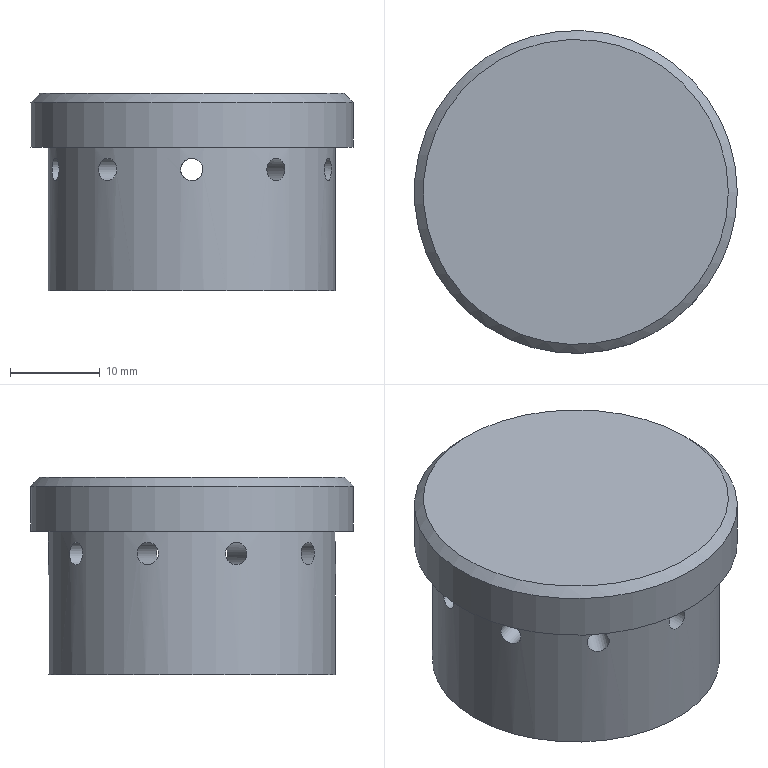Part | NX | features EXTRUDE 12, EXTRACT_STRING 10, Instance Feature 9, DATUM_CSYS 4, SKETCH 3, BOSS 1, CHAMFER 1, CYLINDER 1, Pattern Feature 1 | 1 solid | 20 faces | box 36 x 36 x 22 mm | volume 11377 mm3 | cylinder 14 | plane 5 | cone 1 | commonest cylinder face diameters 2.5 x10 18 x1 25 x1 32 x1 36 x1
STEP:
#1=CARTESIAN_POINT('',(-15.557,-3.74,13.5));
#2=VERTEX_POINT('',#1);
#3=CARTESIAN_POINT('',(-15.496,-4.006,12.519));
#4=CARTESIAN_POINT('',(-15.587,-3.608,13.5));
#5=CARTESIAN_POINT('',(-15.496,-4.006,14.48));
#6=CARTESIAN_POINT('',(-15.229,-4.947,14.885));
#7=CARTESIAN_POINT('',(-14.891,-5.868,14.48));
#8=CARTESIAN_POINT('',(-14.731,-6.243,13.5));
#9=CARTESIAN_POINT('',(-14.891,-5.869,12.522));
#10=CARTESIAN_POINT('',(-15.228,-4.949,12.115));
#11=CARTESIAN_POINT('',(-15.496,-4.006,12.519));
#12=CARTESIAN_POINT('',(-15.587,-3.608,13.5));
#13=CARTESIAN_POINT('',(-15.496,-4.006,14.48));
#14=B_SPLINE_CURVE_WITH_KNOTS('',3,(#3,#4,#5,#6,#7,#8,#9,#10,#11,#12,#13),.UNSPECIFIED.,.T.,.F.,(1,1,1,1,1,1,1,1,1,1,1,1,1,1,1),(-0.002932,-0.001955,-0.0009773,0.,0.0009773,0.001955,0.002932,0.003909,0.004886,0.005864,0.006841,0.007818,0.008795,0.009773,0.01075),.UNSPECIFIED.);
#15=EDGE_CURVE('',#2,#2,#14,.T.);
#16=ORIENTED_EDGE('',*,*,#15,.T.);
#17=EDGE_LOOP('',(#16));
#18=FACE_BOUND('',#17,.T.);
#19=CARTESIAN_POINT('',(-8.365,13.639,13.5));
#20=VERTEX_POINT('',#19);
#21=CARTESIAN_POINT('',(-8.598,13.5,12.519));
#22=CARTESIAN_POINT('',(-8.248,13.709,13.5));
#23=CARTESIAN_POINT('',(-8.598,13.5,14.48));
#24=CARTESIAN_POINT('',(-9.411,12.955,14.885));
#25=CARTESIAN_POINT('',(-10.182,12.349,14.48));
#26=CARTESIAN_POINT('',(-10.489,12.081,13.5));
#27=CARTESIAN_POINT('',(-10.183,12.348,12.522));
#28=CARTESIAN_POINT('',(-9.413,12.953,12.115));
#29=CARTESIAN_POINT('',(-8.598,13.5,12.519));
#30=CARTESIAN_POINT('',(-8.248,13.709,13.5));
#31=CARTESIAN_POINT('',(-8.598,13.5,14.48));
#32=B_SPLINE_CURVE_WITH_KNOTS('',3,(#21,#22,#23,#24,#25,#26,#27,#28,#29,#30,#31),.UNSPECIFIED.,.T.,.F.,(1,1,1,1,1,1,1,1,1,1,1,1,1,1,1),(-0.002932,-0.001955,-0.0009773,0.,0.0009773,0.001955,0.002932,0.003909,0.004886,0.005864,0.006841,0.007818,0.008795,0.009773,0.01075),.UNSPECIFIED.);
#33=EDGE_CURVE('',#20,#20,#32,.T.);
#34=ORIENTED_EDGE('',*,*,#33,.T.);
#35=EDGE_LOOP('',(#34));
#36=FACE_BOUND('',#35,.T.);
#37=CARTESIAN_POINT('',(10.387,12.17,13.5));
#38=VERTEX_POINT('',#37);
#39=CARTESIAN_POINT('',(10.182,12.349,12.519));
#40=CARTESIAN_POINT('',(10.49,12.08,13.5));
#41=CARTESIAN_POINT('',(10.182,12.349,14.48));
#42=CARTESIAN_POINT('',(9.413,12.954,14.885));
#43=CARTESIAN_POINT('',(8.598,13.5,14.48));
#44=CARTESIAN_POINT('',(8.248,13.709,13.5));
#45=CARTESIAN_POINT('',(8.597,13.501,12.522));
#46=CARTESIAN_POINT('',(9.411,12.955,12.115));
#47=CARTESIAN_POINT('',(10.182,12.349,12.519));
#48=CARTESIAN_POINT('',(10.49,12.08,13.5));
#49=CARTESIAN_POINT('',(10.182,12.349,14.48));
#50=B_SPLINE_CURVE_WITH_KNOTS('',3,(#39,#40,#41,#42,#43,#44,#45,#46,#47,#48,#49),.UNSPECIFIED.,.T.,.F.,(1,1,1,1,1,1,1,1,1,1,1,1,1,1,1),(-0.002932,-0.001955,-0.0009773,0.,0.0009773,0.001955,0.002932,0.003909,0.004886,0.005864,0.006841,0.007818,0.008795,0.009773,0.01075),.UNSPECIFIED.);
#51=EDGE_CURVE('',#38,#38,#50,.T.);
#52=ORIENTED_EDGE('',*,*,#51,.T.);
#53=EDGE_LOOP('',(#52));
#54=FACE_BOUND('',#53,.T.);
#55=CARTESIAN_POINT('',(14.784,-6.118,13.5));
#56=VERTEX_POINT('',#55);
#57=CARTESIAN_POINT('',(14.891,-5.868,12.519));
#58=CARTESIAN_POINT('',(14.731,-6.243,13.5));
#59=CARTESIAN_POINT('',(14.891,-5.868,14.48));
#60=CARTESIAN_POINT('',(15.228,-4.949,14.885));
#61=CARTESIAN_POINT('',(15.496,-4.005,14.48));
#62=CARTESIAN_POINT('',(15.587,-3.608,13.5));
#63=CARTESIAN_POINT('',(15.497,-4.004,12.522));
#64=CARTESIAN_POINT('',(15.229,-4.947,12.115));
#65=CARTESIAN_POINT('',(14.891,-5.868,12.519));
#66=CARTESIAN_POINT('',(14.731,-6.243,13.5));
#67=CARTESIAN_POINT('',(14.891,-5.868,14.48));
#68=B_SPLINE_CURVE_WITH_KNOTS('',3,(#57,#58,#59,#60,#61,#62,#63,#64,#65,#66,#67),.UNSPECIFIED.,.T.,.F.,(1,1,1,1,1,1,1,1,1,1,1,1,1,1,1),(-0.002932,-0.001955,-0.0009773,0.,0.0009773,0.001955,0.002932,0.003909,0.004886,0.005864,0.006841,0.007818,0.008795,0.009773,0.01075),.UNSPECIFIED.);
#69=EDGE_CURVE('',#56,#56,#68,.T.);
#70=ORIENTED_EDGE('',*,*,#69,.T.);
#71=EDGE_LOOP('',(#70));
#72=FACE_BOUND('',#71,.T.);
#73=CARTESIAN_POINT('',(0.,-16.,14.75));
#74=VERTEX_POINT('',#73);
#75=CARTESIAN_POINT('',(-0.9806,-15.976,14.479));
#76=CARTESIAN_POINT('',(0.000248,-16.012,14.886));
#77=CARTESIAN_POINT('',(0.9796,-15.976,14.479));
#78=CARTESIAN_POINT('',(1.385,-15.939,13.501));
#79=CARTESIAN_POINT('',(0.9801,-15.976,12.521));
#80=CARTESIAN_POINT('',(0.0002185,-16.012,12.115));
#81=CARTESIAN_POINT('',(-0.9783,-15.976,12.52));
#82=CARTESIAN_POINT('',(-1.385,-15.939,13.499));
#83=CARTESIAN_POINT('',(-0.9806,-15.976,14.479));
#84=CARTESIAN_POINT('',(0.000248,-16.012,14.886));
#85=CARTESIAN_POINT('',(0.9796,-15.976,14.479));
#86=B_SPLINE_CURVE_WITH_KNOTS('',3,(#75,#76,#77,#78,#79,#80,#81,#82,#83,#84,#85),.UNSPECIFIED.,.T.,.F.,(1,1,1,1,1,1,1,1,1,1,1,1,1,1,1),(-0.002932,-0.001955,-0.0009773,0.,0.0009773,0.001955,0.002932,0.003909,0.004886,0.005864,0.006841,0.007818,0.008795,0.009773,0.01075),.UNSPECIFIED.);
#87=EDGE_CURVE('',#74,#74,#86,.T.);
#88=ORIENTED_EDGE('',*,*,#87,.T.);
#89=EDGE_LOOP('',(#88));
#90=FACE_BOUND('',#89,.T.);
#91=CARTESIAN_POINT('',(16.,0.,16.));
#92=VERTEX_POINT('',#91);
#93=CARTESIAN_POINT('',(0.,0.,16.));
#94=DIRECTION('',(0.,0.,-1.));
#95=DIRECTION('',(1.,0.,0.));
#96=AXIS2_PLACEMENT_3D('',#93,#94,#95);
#97=CIRCLE('',#96,16.);
#98=EDGE_CURVE('',#92,#92,#97,.T.);
#99=ORIENTED_EDGE('',*,*,#98,.T.);
#100=EDGE_LOOP('',(#99));
#101=FACE_BOUND('',#100,.T.);
#102=CARTESIAN_POINT('',(16.,0.,0.));
#103=VERTEX_POINT('',#102);
#104=CARTESIAN_POINT('',(0.,0.,0.));
#105=DIRECTION('',(0.,0.,1.));
#106=DIRECTION('',(1.,0.,0.));
#107=AXIS2_PLACEMENT_3D('',#104,#105,#106);
#108=CIRCLE('',#107,16.);
#109=EDGE_CURVE('',#103,#103,#108,.T.);
#110=ORIENTED_EDGE('',*,*,#109,.T.);
#111=EDGE_LOOP('',(#110));
#112=FACE_BOUND('',#111,.T.);
#113=CARTESIAN_POINT('',(8.365,-13.639,13.5));
#114=VERTEX_POINT('',#113);
#115=CARTESIAN_POINT('',(8.598,-13.5,12.519));
#116=CARTESIAN_POINT('',(8.248,-13.709,13.5));
#117=CARTESIAN_POINT('',(8.598,-13.5,14.48));
#118=CARTESIAN_POINT('',(9.411,-12.955,14.885));
#119=CARTESIAN_POINT('',(10.182,-12.349,14.48));
#120=CARTESIAN_POINT('',(10.489,-12.081,13.5));
#121=CARTESIAN_POINT('',(10.183,-12.348,12.522));
#122=CARTESIAN_POINT('',(9.413,-12.953,12.115));
#123=CARTESIAN_POINT('',(8.598,-13.5,12.519));
#124=CARTESIAN_POINT('',(8.248,-13.709,13.5));
#125=CARTESIAN_POINT('',(8.598,-13.5,14.48));
#126=B_SPLINE_CURVE_WITH_KNOTS('',3,(#115,#116,#117,#118,#119,#120,#121,#122,#123,#124,#125),.UNSPECIFIED.,.T.,.F.,(1,1,1,1,1,1,1,1,1,1,1,1,1,1,1),(-0.002932,-0.001955,-0.0009773,0.,0.0009773,0.001955,0.002932,0.003909,0.004886,0.005864,0.006841,0.007818,0.008795,0.009773,0.01075),.UNSPECIFIED.);
#127=EDGE_CURVE('',#114,#114,#126,.T.);
#128=ORIENTED_EDGE('',*,*,#127,.T.);
#129=EDGE_LOOP('',(#128));
#130=FACE_BOUND('',#129,.T.);
#131=CARTESIAN_POINT('',(15.557,3.74,13.5));
#132=VERTEX_POINT('',#131);
#133=CARTESIAN_POINT('',(15.496,4.006,12.519));
#134=CARTESIAN_POINT('',(15.587,3.608,13.5));
#135=CARTESIAN_POINT('',(15.496,4.006,14.48));
#136=CARTESIAN_POINT('',(15.229,4.947,14.885));
#137=CARTESIAN_POINT('',(14.891,5.868,14.48));
#138=CARTESIAN_POINT('',(14.731,6.243,13.5));
#139=CARTESIAN_POINT('',(14.891,5.869,12.522));
#140=CARTESIAN_POINT('',(15.228,4.949,12.115));
#141=CARTESIAN_POINT('',(15.496,4.006,12.519));
#142=CARTESIAN_POINT('',(15.587,3.608,13.5));
#143=CARTESIAN_POINT('',(15.496,4.006,14.48));
#144=B_SPLINE_CURVE_WITH_KNOTS('',3,(#133,#134,#135,#136,#137,#138,#139,#140,#141,#142,#143),.UNSPECIFIED.,.T.,.F.,(1,1,1,1,1,1,1,1,1,1,1,1,1,1,1),(-0.002932,-0.001955,-0.0009773,0.,0.0009773,0.001955,0.002932,0.003909,0.004886,0.005864,0.006841,0.007818,0.008795,0.009773,0.01075),.UNSPECIFIED.);
#145=EDGE_CURVE('',#132,#132,#144,.T.);
#146=ORIENTED_EDGE('',*,*,#145,.T.);
#147=EDGE_LOOP('',(#146));
#148=FACE_BOUND('',#147,.T.);
#149=CARTESIAN_POINT('',(1.25,15.951,13.5));
#150=VERTEX_POINT('',#149);
#151=CARTESIAN_POINT('',(0.9787,15.976,12.519));
#152=CARTESIAN_POINT('',(1.386,15.939,13.5));
#153=CARTESIAN_POINT('',(0.979,15.976,14.48));
#154=CARTESIAN_POINT('',(0.001053,16.012,14.885));
#155=CARTESIAN_POINT('',(-0.9792,15.976,14.48));
#156=CARTESIAN_POINT('',(-1.385,15.939,13.5));
#157=CARTESIAN_POINT('',(-0.9805,15.976,12.522));
#158=CARTESIAN_POINT('',(-0.001401,16.012,12.115));
#159=CARTESIAN_POINT('',(0.9787,15.976,12.519));
#160=CARTESIAN_POINT('',(1.386,15.939,13.5));
#161=CARTESIAN_POINT('',(0.979,15.976,14.48));
#162=B_SPLINE_CURVE_WITH_KNOTS('',3,(#151,#152,#153,#154,#155,#156,#157,#158,#159,#160,#161),.UNSPECIFIED.,.T.,.F.,(1,1,1,1,1,1,1,1,1,1,1,1,1,1,1),(-0.002932,-0.001955,-0.0009773,0.,0.0009773,0.001955,0.002932,0.003909,0.004886,0.005864,0.006841,0.007818,0.008795,0.009773,0.01075),.UNSPECIFIED.);
#163=EDGE_CURVE('',#150,#150,#162,.T.);
#164=ORIENTED_EDGE('',*,*,#163,.T.);
#165=EDGE_LOOP('',(#164));
#166=FACE_BOUND('',#165,.T.);
#167=CARTESIAN_POINT('',(-14.784,6.118,13.5));
#168=VERTEX_POINT('',#167);
#169=CARTESIAN_POINT('',(-14.891,5.868,12.519));
#170=CARTESIAN_POINT('',(-14.731,6.243,13.5));
#171=CARTESIAN_POINT('',(-14.891,5.868,14.48));
#172=CARTESIAN_POINT('',(-15.228,4.949,14.885));
#173=CARTESIAN_POINT('',(-15.496,4.005,14.48));
#174=CARTESIAN_POINT('',(-15.587,3.608,13.5));
#175=CARTESIAN_POINT('',(-15.497,4.004,12.522));
#176=CARTESIAN_POINT('',(-15.229,4.947,12.115));
#177=CARTESIAN_POINT('',(-14.891,5.868,12.519));
#178=CARTESIAN_POINT('',(-14.731,6.243,13.5));
#179=CARTESIAN_POINT('',(-14.891,5.868,14.48));
#180=B_SPLINE_CURVE_WITH_KNOTS('',3,(#169,#170,#171,#172,#173,#174,#175,#176,#177,#178,#179),.UNSPECIFIED.,.T.,.F.,(1,1,1,1,1,1,1,1,1,1,1,1,1,1,1),(-0.002932,-0.001955,-0.0009773,0.,0.0009773,0.001955,0.002932,0.003909,0.004886,0.005864,0.006841,0.007818,0.008795,0.009773,0.01075),.UNSPECIFIED.);
#181=EDGE_CURVE('',#168,#168,#180,.T.);
#182=ORIENTED_EDGE('',*,*,#181,.T.);
#183=EDGE_LOOP('',(#182));
#184=FACE_BOUND('',#183,.T.);
#185=CARTESIAN_POINT('',(-10.387,-12.17,13.5));
#186=VERTEX_POINT('',#185);
#187=CARTESIAN_POINT('',(-10.182,-12.349,12.519));
#188=CARTESIAN_POINT('',(-10.49,-12.08,13.5));
#189=CARTESIAN_POINT('',(-10.182,-12.349,14.48));
#190=CARTESIAN_POINT('',(-9.413,-12.954,14.885));
#191=CARTESIAN_POINT('',(-8.598,-13.5,14.48));
#192=CARTESIAN_POINT('',(-8.248,-13.709,13.5));
#193=CARTESIAN_POINT('',(-8.597,-13.501,12.522));
#194=CARTESIAN_POINT('',(-9.411,-12.955,12.115));
#195=CARTESIAN_POINT('',(-10.182,-12.349,12.519));
#196=CARTESIAN_POINT('',(-10.49,-12.08,13.5));
#197=CARTESIAN_POINT('',(-10.182,-12.349,14.48));
#198=B_SPLINE_CURVE_WITH_KNOTS('',3,(#187,#188,#189,#190,#191,#192,#193,#194,#195,#196,#197),.UNSPECIFIED.,.T.,.F.,(1,1,1,1,1,1,1,1,1,1,1,1,1,1,1),(-0.002932,-0.001955,-0.0009773,0.,0.0009773,0.001955,0.002932,0.003909,0.004886,0.005864,0.006841,0.007818,0.008795,0.009773,0.01075),.UNSPECIFIED.);
#199=EDGE_CURVE('',#186,#186,#198,.T.);
#200=ORIENTED_EDGE('',*,*,#199,.T.);
#201=EDGE_LOOP('',(#200));
#202=FACE_BOUND('',#201,.T.);
#203=CARTESIAN_POINT('',(0.,0.,0.));
#204=DIRECTION('',(0.,0.,1.));
#205=DIRECTION('',(1.,0.,0.));
#206=AXIS2_PLACEMENT_3D('',#203,#204,#205);
#207=CYLINDRICAL_SURFACE('',#206,16.);
#208=ADVANCED_FACE('',(#18,#36,#54,#72,#90,#101,#112,#130,#148,#166,#184,#202),#207,.T.);
#209=CARTESIAN_POINT('',(-8.863,-1.565,13.5));
#210=VERTEX_POINT('',#209);
#211=CARTESIAN_POINT('',(-8.821,-1.837,14.481));
#212=CARTESIAN_POINT('',(-8.884,-1.43,13.5));
#213=CARTESIAN_POINT('',(-8.821,-1.837,12.52));
#214=CARTESIAN_POINT('',(-8.58,-2.787,12.115));
#215=CARTESIAN_POINT('',(-8.216,-3.699,12.52));
#216=CARTESIAN_POINT('',(-8.028,-4.065,13.5));
#217=CARTESIAN_POINT('',(-8.215,-3.7,14.478));
#218=CARTESIAN_POINT('',(-8.58,-2.789,14.885));
#219=CARTESIAN_POINT('',(-8.821,-1.837,14.481));
#220=CARTESIAN_POINT('',(-8.884,-1.43,13.5));
#221=CARTESIAN_POINT('',(-8.821,-1.837,12.52));
#222=B_SPLINE_CURVE_WITH_KNOTS('',3,(#211,#212,#213,#214,#215,#216,#217,#218,#219,#220,#221),.UNSPECIFIED.,.T.,.F.,(1,1,1,1,1,1,1,1,1,1,1,1,1,1,1),(-0.002934,-0.001956,-0.0009781,0.,0.0009781,0.001956,0.002934,0.003912,0.00489,0.005868,0.006847,0.007825,0.008803,0.009781,0.01076),.UNSPECIFIED.);
#223=EDGE_CURVE('',#210,#210,#222,.T.);
#224=ORIENTED_EDGE('',*,*,#223,.T.);
#225=EDGE_LOOP('',(#224));
#226=FACE_BOUND('',#225,.T.);
#227=CARTESIAN_POINT('',(-4.228,7.945,13.5));
#228=VERTEX_POINT('',#227);
#229=CARTESIAN_POINT('',(-4.473,7.821,14.481));
#230=CARTESIAN_POINT('',(-4.105,8.007,13.5));
#231=CARTESIAN_POINT('',(-4.473,7.822,12.52));
#232=CARTESIAN_POINT('',(-5.302,7.299,12.115));
#233=CARTESIAN_POINT('',(-6.057,6.67,12.52));
#234=CARTESIAN_POINT('',(-6.346,6.379,13.5));
#235=CARTESIAN_POINT('',(-6.058,6.67,14.478));
#236=CARTESIAN_POINT('',(-5.304,7.298,14.885));
#237=CARTESIAN_POINT('',(-4.473,7.821,14.481));
#238=CARTESIAN_POINT('',(-4.105,8.007,13.5));
#239=CARTESIAN_POINT('',(-4.473,7.822,12.52));
#240=B_SPLINE_CURVE_WITH_KNOTS('',3,(#229,#230,#231,#232,#233,#234,#235,#236,#237,#238,#239),.UNSPECIFIED.,.T.,.F.,(1,1,1,1,1,1,1,1,1,1,1,1,1,1,1),(-0.002934,-0.001956,-0.0009781,0.,0.0009781,0.001956,0.002934,0.003912,0.00489,0.005868,0.006847,0.007825,0.008803,0.009781,0.01076),.UNSPECIFIED.);
#241=EDGE_CURVE('',#228,#228,#240,.T.);
#242=ORIENTED_EDGE('',*,*,#241,.T.);
#243=EDGE_LOOP('',(#242));
#244=FACE_BOUND('',#243,.T.);
#245=CARTESIAN_POINT('',(6.25,6.476,13.5));
#246=VERTEX_POINT('',#245);
#247=CARTESIAN_POINT('',(6.056,6.671,14.481));
#248=CARTESIAN_POINT('',(6.347,6.378,13.5));
#249=CARTESIAN_POINT('',(6.057,6.671,12.52));
#250=CARTESIAN_POINT('',(5.304,7.298,12.115));
#251=CARTESIAN_POINT('',(4.472,7.822,12.52));
#252=CARTESIAN_POINT('',(4.105,8.007,13.5));
#253=CARTESIAN_POINT('',(4.471,7.822,14.478));
#254=CARTESIAN_POINT('',(5.302,7.299,14.885));
#255=CARTESIAN_POINT('',(6.056,6.671,14.481));
#256=CARTESIAN_POINT('',(6.347,6.378,13.5));
#257=CARTESIAN_POINT('',(6.057,6.671,12.52));
#258=B_SPLINE_CURVE_WITH_KNOTS('',3,(#247,#248,#249,#250,#251,#252,#253,#254,#255,#256,#257),.UNSPECIFIED.,.T.,.F.,(1,1,1,1,1,1,1,1,1,1,1,1,1,1,1),(-0.002934,-0.001956,-0.0009781,0.,0.0009781,0.001956,0.002934,0.003912,0.00489,0.005868,0.006847,0.007825,0.008803,0.009781,0.01076),.UNSPECIFIED.);
#259=EDGE_CURVE('',#246,#246,#258,.T.);
#260=ORIENTED_EDGE('',*,*,#259,.T.);
#261=EDGE_LOOP('',(#260));
#262=FACE_BOUND('',#261,.T.);
#263=CARTESIAN_POINT('',(8.09,-3.943,13.5));
#264=VERTEX_POINT('',#263);
#265=CARTESIAN_POINT('',(8.216,-3.699,14.481));
#266=CARTESIAN_POINT('',(8.028,-4.065,13.5));
#267=CARTESIAN_POINT('',(8.216,-3.699,12.52));
#268=CARTESIAN_POINT('',(8.58,-2.789,12.115));
#269=CARTESIAN_POINT('',(8.821,-1.836,12.52));
#270=CARTESIAN_POINT('',(8.884,-1.43,13.5));
#271=CARTESIAN_POINT('',(8.821,-1.835,14.478));
#272=CARTESIAN_POINT('',(8.581,-2.787,14.885));
#273=CARTESIAN_POINT('',(8.216,-3.699,14.481));
#274=CARTESIAN_POINT('',(8.028,-4.065,13.5));
#275=CARTESIAN_POINT('',(8.216,-3.699,12.52));
#276=B_SPLINE_CURVE_WITH_KNOTS('',3,(#265,#266,#267,#268,#269,#270,#271,#272,#273,#274,#275),.UNSPECIFIED.,.T.,.F.,(1,1,1,1,1,1,1,1,1,1,1,1,1,1,1),(-0.002934,-0.001956,-0.0009781,0.,0.0009781,0.001956,0.002934,0.003912,0.00489,0.005868,0.006847,0.007825,0.008803,0.009781,0.01076),.UNSPECIFIED.);
#277=EDGE_CURVE('',#264,#264,#276,.T.);
#278=ORIENTED_EDGE('',*,*,#277,.T.);
#279=EDGE_LOOP('',(#278));
#280=FACE_BOUND('',#279,.T.);
#281=CARTESIAN_POINT('',(0.,-9.,14.75));
#282=VERTEX_POINT('',#281);
#283=CARTESIAN_POINT('',(0.9806,-8.956,14.479));
#284=CARTESIAN_POINT('',(-0.0002391,-9.022,14.886));
#285=CARTESIAN_POINT('',(-0.9796,-8.957,14.479));
#286=CARTESIAN_POINT('',(-1.385,-8.891,13.501));
#287=CARTESIAN_POINT('',(-0.98,-8.957,12.521));
#288=CARTESIAN_POINT('',(-0.0003086,-9.022,12.115));
#289=CARTESIAN_POINT('',(0.9783,-8.957,12.519));
#290=CARTESIAN_POINT('',(1.385,-8.891,13.499));
#291=CARTESIAN_POINT('',(0.9806,-8.956,14.479));
#292=CARTESIAN_POINT('',(-0.0002391,-9.022,14.886));
#293=CARTESIAN_POINT('',(-0.9796,-8.957,14.479));
#294=B_SPLINE_CURVE_WITH_KNOTS('',3,(#283,#284,#285,#286,#287,#288,#289,#290,#291,#292,#293),.UNSPECIFIED.,.T.,.F.,(1,1,1,1,1,1,1,1,1,1,1,1,1,1,1),(-0.002934,-0.001956,-0.0009781,0.,0.0009781,0.001956,0.002934,0.003912,0.00489,0.005868,0.006847,0.007825,0.008803,0.009781,0.01076),.UNSPECIFIED.);
#295=EDGE_CURVE('',#282,#282,#294,.T.);
#296=ORIENTED_EDGE('',*,*,#295,.T.);
#297=EDGE_LOOP('',(#296));
#298=FACE_BOUND('',#297,.T.);
#299=CARTESIAN_POINT('',(9.,0.,19.));
#300=VERTEX_POINT('',#299);
#301=CARTESIAN_POINT('',(0.,0.,19.));
#302=DIRECTION('',(0.,0.,1.));
#303=DIRECTION('',(1.,0.,0.));
#304=AXIS2_PLACEMENT_3D('',#301,#302,#303);
#305=CIRCLE('',#304,9.);
#306=EDGE_CURVE('',#300,#300,#305,.F.);
#307=ORIENTED_EDGE('',*,*,#306,.F.);
#308=EDGE_LOOP('',(#307));
#309=FACE_BOUND('',#308,.T.);
#310=CARTESIAN_POINT('',(9.,0.,10.));
#311=VERTEX_POINT('',#310);
#312=CARTESIAN_POINT('',(0.,0.,10.));
#313=DIRECTION('',(0.,0.,1.));
#314=DIRECTION('',(1.,0.,0.));
#315=AXIS2_PLACEMENT_3D('',#312,#313,#314);
#316=CIRCLE('',#315,9.);
#317=EDGE_CURVE('',#311,#311,#316,.T.);
#318=ORIENTED_EDGE('',*,*,#317,.F.);
#319=EDGE_LOOP('',(#318));
#320=FACE_BOUND('',#319,.T.);
#321=CARTESIAN_POINT('',(4.228,-7.945,13.5));
#322=VERTEX_POINT('',#321);
#323=CARTESIAN_POINT('',(4.473,-7.821,14.481));
#324=CARTESIAN_POINT('',(4.105,-8.007,13.5));
#325=CARTESIAN_POINT('',(4.473,-7.822,12.52));
#326=CARTESIAN_POINT('',(5.302,-7.299,12.115));
#327=CARTESIAN_POINT('',(6.057,-6.67,12.52));
#328=CARTESIAN_POINT('',(6.346,-6.379,13.5));
#329=CARTESIAN_POINT('',(6.058,-6.67,14.478));
#330=CARTESIAN_POINT('',(5.304,-7.298,14.885));
#331=CARTESIAN_POINT('',(4.473,-7.821,14.481));
#332=CARTESIAN_POINT('',(4.105,-8.007,13.5));
#333=CARTESIAN_POINT('',(4.473,-7.822,12.52));
#334=B_SPLINE_CURVE_WITH_KNOTS('',3,(#323,#324,#325,#326,#327,#328,#329,#330,#331,#332,#333),.UNSPECIFIED.,.T.,.F.,(1,1,1,1,1,1,1,1,1,1,1,1,1,1,1),(-0.002934,-0.001956,-0.0009781,0.,0.0009781,0.001956,0.002934,0.003912,0.00489,0.005868,0.006847,0.007825,0.008803,0.009781,0.01076),.UNSPECIFIED.);
#335=EDGE_CURVE('',#322,#322,#334,.T.);
#336=ORIENTED_EDGE('',*,*,#335,.T.);
#337=EDGE_LOOP('',(#336));
#338=FACE_BOUND('',#337,.T.);
#339=CARTESIAN_POINT('',(8.863,1.565,13.5));
#340=VERTEX_POINT('',#339);
#341=CARTESIAN_POINT('',(8.821,1.837,14.481));
#342=CARTESIAN_POINT('',(8.884,1.43,13.5));
#343=CARTESIAN_POINT('',(8.821,1.837,12.52));
#344=CARTESIAN_POINT('',(8.58,2.787,12.115));
#345=CARTESIAN_POINT('',(8.216,3.699,12.52));
#346=CARTESIAN_POINT('',(8.028,4.065,13.5));
#347=CARTESIAN_POINT('',(8.215,3.7,14.478));
#348=CARTESIAN_POINT('',(8.58,2.789,14.885));
#349=CARTESIAN_POINT('',(8.821,1.837,14.481));
#350=CARTESIAN_POINT('',(8.884,1.43,13.5));
#351=CARTESIAN_POINT('',(8.821,1.837,12.52));
#352=B_SPLINE_CURVE_WITH_KNOTS('',3,(#341,#342,#343,#344,#345,#346,#347,#348,#349,#350,#351),.UNSPECIFIED.,.T.,.F.,(1,1,1,1,1,1,1,1,1,1,1,1,1,1,1),(-0.002934,-0.001956,-0.0009781,0.,0.0009781,0.001956,0.002934,0.003912,0.00489,0.005868,0.006847,0.007825,0.008803,0.009781,0.01076),.UNSPECIFIED.);
#353=EDGE_CURVE('',#340,#340,#352,.T.);
#354=ORIENTED_EDGE('',*,*,#353,.T.);
#355=EDGE_LOOP('',(#354));
#356=FACE_BOUND('',#355,.T.);
#357=CARTESIAN_POINT('',(1.25,8.913,13.5));
#358=VERTEX_POINT('',#357);
#359=CARTESIAN_POINT('',(0.9787,8.957,14.481));
#360=CARTESIAN_POINT('',(1.386,8.891,13.5));
#361=CARTESIAN_POINT('',(0.979,8.957,12.52));
#362=CARTESIAN_POINT('',(0.001148,9.022,12.115));
#363=CARTESIAN_POINT('',(-0.9794,8.957,12.52));
#364=CARTESIAN_POINT('',(-1.385,8.891,13.5));
#365=CARTESIAN_POINT('',(-0.9805,8.956,14.478));
#366=CARTESIAN_POINT('',(-0.00118,9.022,14.885));
#367=CARTESIAN_POINT('',(0.9787,8.957,14.481));
#368=CARTESIAN_POINT('',(1.386,8.891,13.5));
#369=CARTESIAN_POINT('',(0.979,8.957,12.52));
#370=B_SPLINE_CURVE_WITH_KNOTS('',3,(#359,#360,#361,#362,#363,#364,#365,#366,#367,#368,#369),.UNSPECIFIED.,.T.,.F.,(1,1,1,1,1,1,1,1,1,1,1,1,1,1,1),(-0.002934,-0.001956,-0.0009781,0.,0.0009781,0.001956,0.002934,0.003912,0.00489,0.005868,0.006847,0.007825,0.008803,0.009781,0.01076),.UNSPECIFIED.);
#371=EDGE_CURVE('',#358,#358,#370,.T.);
#372=ORIENTED_EDGE('',*,*,#371,.T.);
#373=EDGE_LOOP('',(#372));
#374=FACE_BOUND('',#373,.T.);
#375=CARTESIAN_POINT('',(-8.09,3.943,13.5));
#376=VERTEX_POINT('',#375);
#377=CARTESIAN_POINT('',(-8.216,3.699,14.481));
#378=CARTESIAN_POINT('',(-8.028,4.065,13.5));
#379=CARTESIAN_POINT('',(-8.216,3.699,12.52));
#380=CARTESIAN_POINT('',(-8.58,2.789,12.115));
#381=CARTESIAN_POINT('',(-8.821,1.836,12.52));
#382=CARTESIAN_POINT('',(-8.884,1.43,13.5));
#383=CARTESIAN_POINT('',(-8.821,1.835,14.478));
#384=CARTESIAN_POINT('',(-8.581,2.787,14.885));
#385=CARTESIAN_POINT('',(-8.216,3.699,14.481));
#386=CARTESIAN_POINT('',(-8.028,4.065,13.5));
#387=CARTESIAN_POINT('',(-8.216,3.699,12.52));
#388=B_SPLINE_CURVE_WITH_KNOTS('',3,(#377,#378,#379,#380,#381,#382,#383,#384,#385,#386,#387),.UNSPECIFIED.,.T.,.F.,(1,1,1,1,1,1,1,1,1,1,1,1,1,1,1),(-0.002934,-0.001956,-0.0009781,0.,0.0009781,0.001956,0.002934,0.003912,0.00489,0.005868,0.006847,0.007825,0.008803,0.009781,0.01076),.UNSPECIFIED.);
#389=EDGE_CURVE('',#376,#376,#388,.T.);
#390=ORIENTED_EDGE('',*,*,#389,.T.);
#391=EDGE_LOOP('',(#390));
#392=FACE_BOUND('',#391,.T.);
#393=CARTESIAN_POINT('',(-6.25,-6.476,13.5));
#394=VERTEX_POINT('',#393);
#395=CARTESIAN_POINT('',(-6.056,-6.671,14.481));
#396=CARTESIAN_POINT('',(-6.347,-6.378,13.5));
#397=CARTESIAN_POINT('',(-6.057,-6.671,12.52));
#398=CARTESIAN_POINT('',(-5.304,-7.298,12.115));
#399=CARTESIAN_POINT('',(-4.472,-7.822,12.52));
#400=CARTESIAN_POINT('',(-4.105,-8.007,13.5));
#401=CARTESIAN_POINT('',(-4.471,-7.822,14.478));
#402=CARTESIAN_POINT('',(-5.302,-7.299,14.885));
#403=CARTESIAN_POINT('',(-6.056,-6.671,14.481));
#404=CARTESIAN_POINT('',(-6.347,-6.378,13.5));
#405=CARTESIAN_POINT('',(-6.057,-6.671,12.52));
#406=B_SPLINE_CURVE_WITH_KNOTS('',3,(#395,#396,#397,#398,#399,#400,#401,#402,#403,#404,#405),.UNSPECIFIED.,.T.,.F.,(1,1,1,1,1,1,1,1,1,1,1,1,1,1,1),(-0.002934,-0.001956,-0.0009781,0.,0.0009781,0.001956,0.002934,0.003912,0.00489,0.005868,0.006847,0.007825,0.008803,0.009781,0.01076),.UNSPECIFIED.);
#407=EDGE_CURVE('',#394,#394,#406,.T.);
#408=ORIENTED_EDGE('',*,*,#407,.T.);
#409=EDGE_LOOP('',(#408));
#410=FACE_BOUND('',#409,.T.);
#411=CARTESIAN_POINT('',(0.,0.,19.));
#412=DIRECTION('',(0.,0.,-1.));
#413=DIRECTION('',(-1.,0.,0.));
#414=AXIS2_PLACEMENT_3D('',#411,#412,#413);
#415=CYLINDRICAL_SURFACE('',#414,9.);
#416=ADVANCED_FACE('',(#226,#244,#262,#280,#298,#309,#320,#338,#356,#374,#392,#410),#415,.F.);
#417=CARTESIAN_POINT('',(12.5,0.,0.));
#418=VERTEX_POINT('',#417);
#419=CARTESIAN_POINT('',(0.,0.,0.));
#420=DIRECTION('',(0.,0.,1.));
#421=DIRECTION('',(1.,0.,0.));
#422=AXIS2_PLACEMENT_3D('',#419,#420,#421);
#423=CIRCLE('',#422,12.5);
#424=EDGE_CURVE('',#418,#418,#423,.T.);
#425=ORIENTED_EDGE('',*,*,#424,.T.);
#426=EDGE_LOOP('',(#425));
#427=FACE_BOUND('',#426,.T.);
#428=ORIENTED_EDGE('',*,*,#109,.F.);
#429=EDGE_LOOP('',(#428));
#430=FACE_BOUND('',#429,.T.);
#431=CARTESIAN_POINT('',(0.,0.,0.));
#432=DIRECTION('',(0.,0.,-1.));
#433=DIRECTION('',(-1.,0.,0.));
#434=AXIS2_PLACEMENT_3D('',#431,#432,#433);
#435=PLANE('',#434);
#436=ADVANCED_FACE('',(#427,#430),#435,.T.);
#437=CARTESIAN_POINT('',(17.,0.,22.));
#438=VERTEX_POINT('',#437);
#439=CARTESIAN_POINT('',(0.,0.,22.));
#440=DIRECTION('',(0.,0.,1.));
#441=DIRECTION('',(1.,0.,0.));
#442=AXIS2_PLACEMENT_3D('',#439,#440,#441);
#443=CIRCLE('',#442,17.);
#444=EDGE_CURVE('',#438,#438,#443,.T.);
#445=ORIENTED_EDGE('',*,*,#444,.T.);
#446=EDGE_LOOP('',(#445));
#447=FACE_BOUND('',#446,.T.);
#448=CARTESIAN_POINT('',(0.,0.,22.));
#449=DIRECTION('',(0.,0.,1.));
#450=DIRECTION('',(1.,0.,0.));
#451=AXIS2_PLACEMENT_3D('',#448,#449,#450);
#452=PLANE('',#451);
#453=ADVANCED_FACE('',(#447),#452,.T.);
#454=ORIENTED_EDGE('',*,*,#98,.F.);
#455=EDGE_LOOP('',(#454));
#456=FACE_BOUND('',#455,.T.);
#457=CARTESIAN_POINT('',(18.,0.,16.));
#458=VERTEX_POINT('',#457);
#459=CARTESIAN_POINT('',(0.,0.,16.));
#460=DIRECTION('',(0.,0.,1.));
#461=DIRECTION('',(1.,0.,0.));
#462=AXIS2_PLACEMENT_3D('',#459,#460,#461);
#463=CIRCLE('',#462,18.);
#464=EDGE_CURVE('',#458,#458,#463,.T.);
#465=ORIENTED_EDGE('',*,*,#464,.F.);
#466=EDGE_LOOP('',(#465));
#467=FACE_BOUND('',#466,.T.);
#468=CARTESIAN_POINT('',(0.,0.,16.));
#469=DIRECTION('',(0.,0.,-1.));
#470=DIRECTION('',(-1.,0.,0.));
#471=AXIS2_PLACEMENT_3D('',#468,#469,#470);
#472=PLANE('',#471);
#473=ADVANCED_FACE('',(#456,#467),#472,.T.);
#474=CARTESIAN_POINT('',(18.,0.,21.));
#475=VERTEX_POINT('',#474);
#476=CARTESIAN_POINT('',(0.,0.,21.));
#477=DIRECTION('',(0.,0.,1.));
#478=DIRECTION('',(1.,0.,0.));
#479=AXIS2_PLACEMENT_3D('',#476,#477,#478);
#480=CIRCLE('',#479,18.);
#481=EDGE_CURVE('',#475,#475,#480,.F.);
#482=ORIENTED_EDGE('',*,*,#481,.T.);
#483=EDGE_LOOP('',(#482));
#484=FACE_BOUND('',#483,.T.);
#485=ORIENTED_EDGE('',*,*,#464,.T.);
#486=EDGE_LOOP('',(#485));
#487=FACE_BOUND('',#486,.T.);
#488=CARTESIAN_POINT('',(0.,0.,16.));
#489=DIRECTION('',(0.,0.,1.));
#490=DIRECTION('',(1.,0.,0.));
#491=AXIS2_PLACEMENT_3D('',#488,#489,#490);
#492=CYLINDRICAL_SURFACE('',#491,18.);
#493=ADVANCED_FACE('',(#484,#487),#492,.T.);
#494=CARTESIAN_POINT('',(12.5,0.,10.));
#495=VERTEX_POINT('',#494);
#496=CARTESIAN_POINT('',(0.,0.,10.));
#497=DIRECTION('',(0.,0.,1.));
#498=DIRECTION('',(1.,0.,0.));
#499=AXIS2_PLACEMENT_3D('',#496,#497,#498);
#500=CIRCLE('',#499,12.5);
#501=EDGE_CURVE('',#495,#495,#500,.F.);
#502=ORIENTED_EDGE('',*,*,#501,.F.);
#503=EDGE_LOOP('',(#502));
#504=FACE_BOUND('',#503,.T.);
#505=ORIENTED_EDGE('',*,*,#424,.F.);
#506=EDGE_LOOP('',(#505));
#507=FACE_BOUND('',#506,.T.);
#508=CARTESIAN_POINT('',(0.,0.,10.));
#509=DIRECTION('',(0.,0.,-1.));
#510=DIRECTION('',(-1.,0.,0.));
#511=AXIS2_PLACEMENT_3D('',#508,#509,#510);
#512=CYLINDRICAL_SURFACE('',#511,12.5);
#513=ADVANCED_FACE('',(#504,#507),#512,.F.);
#514=ORIENTED_EDGE('',*,*,#317,.T.);
#515=EDGE_LOOP('',(#514));
#516=FACE_BOUND('',#515,.T.);
#517=ORIENTED_EDGE('',*,*,#501,.T.);
#518=EDGE_LOOP('',(#517));
#519=FACE_BOUND('',#518,.T.);
#520=CARTESIAN_POINT('',(0.,0.,10.));
#521=DIRECTION('',(0.,0.,1.));
#522=DIRECTION('',(1.,0.,0.));
#523=AXIS2_PLACEMENT_3D('',#520,#521,#522);
#524=PLANE('',#523);
#525=ADVANCED_FACE('',(#516,#519),#524,.F.);
#526=ORIENTED_EDGE('',*,*,#306,.T.);
#527=EDGE_LOOP('',(#526));
#528=FACE_BOUND('',#527,.T.);
#529=CARTESIAN_POINT('',(0.,0.,19.));
#530=DIRECTION('',(0.,0.,1.));
#531=DIRECTION('',(1.,0.,0.));
#532=AXIS2_PLACEMENT_3D('',#529,#530,#531);
#533=PLANE('',#532);
#534=ADVANCED_FACE('',(#528),#533,.F.);
#535=ORIENTED_EDGE('',*,*,#481,.F.);
#536=EDGE_LOOP('',(#535));
#537=FACE_BOUND('',#536,.T.);
#538=ORIENTED_EDGE('',*,*,#444,.F.);
#539=EDGE_LOOP('',(#538));
#540=FACE_BOUND('',#539,.T.);
#541=CARTESIAN_POINT('',(0.,0.,22.));
#542=DIRECTION('',(0.,0.,-1.));
#543=DIRECTION('',(-1.,0.,0.));
#544=AXIS2_PLACEMENT_3D('',#541,#542,#543);
#545=CONICAL_SURFACE('',#544,17.,0.7854);
#546=ADVANCED_FACE('',(#537,#540),#545,.T.);
#547=ORIENTED_EDGE('',*,*,#87,.F.);
#548=EDGE_LOOP('',(#547));
#549=FACE_BOUND('',#548,.T.);
#550=ORIENTED_EDGE('',*,*,#295,.F.);
#551=EDGE_LOOP('',(#550));
#552=FACE_BOUND('',#551,.T.);
#553=CARTESIAN_POINT('',(0.,-19.5,13.5));
#554=DIRECTION('',(0.,1.,0.));
#555=DIRECTION('',(0.,0.,1.));
#556=AXIS2_PLACEMENT_3D('',#553,#554,#555);
#557=CYLINDRICAL_SURFACE('',#556,1.25);
#558=ADVANCED_FACE('',(#549,#552),#557,.F.);
#559=ORIENTED_EDGE('',*,*,#127,.F.);
#560=EDGE_LOOP('',(#559));
#561=FACE_BOUND('',#560,.T.);
#562=ORIENTED_EDGE('',*,*,#335,.F.);
#563=EDGE_LOOP('',(#562));
#564=FACE_BOUND('',#563,.T.);
#565=CARTESIAN_POINT('',(11.462,-15.776,13.5));
#566=DIRECTION('',(-0.5878,0.809,0.));
#567=DIRECTION('',(-0.809,-0.5878,0.));
#568=AXIS2_PLACEMENT_3D('',#565,#566,#567);
#569=CYLINDRICAL_SURFACE('',#568,1.25);
#570=ADVANCED_FACE('',(#561,#564),#569,.F.);
#571=ORIENTED_EDGE('',*,*,#69,.F.);
#572=EDGE_LOOP('',(#571));
#573=FACE_BOUND('',#572,.T.);
#574=ORIENTED_EDGE('',*,*,#277,.F.);
#575=EDGE_LOOP('',(#574));
#576=FACE_BOUND('',#575,.T.);
#577=CARTESIAN_POINT('',(18.546,-6.026,13.5));
#578=DIRECTION('',(-0.9511,0.309,0.));
#579=DIRECTION('',(-0.309,-0.9511,0.));
#580=AXIS2_PLACEMENT_3D('',#577,#578,#579);
#581=CYLINDRICAL_SURFACE('',#580,1.25);
#582=ADVANCED_FACE('',(#573,#576),#581,.F.);
#583=ORIENTED_EDGE('',*,*,#145,.F.);
#584=EDGE_LOOP('',(#583));
#585=FACE_BOUND('',#584,.T.);
#586=ORIENTED_EDGE('',*,*,#353,.F.);
#587=EDGE_LOOP('',(#586));
#588=FACE_BOUND('',#587,.T.);
#589=CARTESIAN_POINT('',(18.546,6.026,13.5));
#590=DIRECTION('',(-0.9511,-0.309,0.));
#591=DIRECTION('',(0.309,-0.9511,0.));
#592=AXIS2_PLACEMENT_3D('',#589,#590,#591);
#593=CYLINDRICAL_SURFACE('',#592,1.25);
#594=ADVANCED_FACE('',(#585,#588),#593,.F.);
#595=ORIENTED_EDGE('',*,*,#51,.F.);
#596=EDGE_LOOP('',(#595));
#597=FACE_BOUND('',#596,.T.);
#598=ORIENTED_EDGE('',*,*,#259,.F.);
#599=EDGE_LOOP('',(#598));
#600=FACE_BOUND('',#599,.T.);
#601=CARTESIAN_POINT('',(11.462,15.776,13.5));
#602=DIRECTION('',(-0.5878,-0.809,0.));
#603=DIRECTION('',(0.809,-0.5878,0.));
#604=AXIS2_PLACEMENT_3D('',#601,#602,#603);
#605=CYLINDRICAL_SURFACE('',#604,1.25);
#606=ADVANCED_FACE('',(#597,#600),#605,.F.);
#607=ORIENTED_EDGE('',*,*,#163,.F.);
#608=EDGE_LOOP('',(#607));
#609=FACE_BOUND('',#608,.T.);
#610=ORIENTED_EDGE('',*,*,#371,.F.);
#611=EDGE_LOOP('',(#610));
#612=FACE_BOUND('',#611,.T.);
#613=CARTESIAN_POINT('',(0.,19.5,13.5));
#614=DIRECTION('',(0.,-1.,0.));
#615=DIRECTION('',(1.,0.,0.));
#616=AXIS2_PLACEMENT_3D('',#613,#614,#615);
#617=CYLINDRICAL_SURFACE('',#616,1.25);
#618=ADVANCED_FACE('',(#609,#612),#617,.F.);
#619=ORIENTED_EDGE('',*,*,#33,.F.);
#620=EDGE_LOOP('',(#619));
#621=FACE_BOUND('',#620,.T.);
#622=ORIENTED_EDGE('',*,*,#241,.F.);
#623=EDGE_LOOP('',(#622));
#624=FACE_BOUND('',#623,.T.);
#625=CARTESIAN_POINT('',(-11.462,15.776,13.5));
#626=DIRECTION('',(0.5878,-0.809,0.));
#627=DIRECTION('',(0.809,0.5878,0.));
#628=AXIS2_PLACEMENT_3D('',#625,#626,#627);
#629=CYLINDRICAL_SURFACE('',#628,1.25);
#630=ADVANCED_FACE('',(#621,#624),#629,.F.);
#631=ORIENTED_EDGE('',*,*,#181,.F.);
#632=EDGE_LOOP('',(#631));
#633=FACE_BOUND('',#632,.T.);
#634=ORIENTED_EDGE('',*,*,#389,.F.);
#635=EDGE_LOOP('',(#634));
#636=FACE_BOUND('',#635,.T.);
#637=CARTESIAN_POINT('',(-18.546,6.026,13.5));
#638=DIRECTION('',(0.9511,-0.309,0.));
#639=DIRECTION('',(0.309,0.9511,0.));
#640=AXIS2_PLACEMENT_3D('',#637,#638,#639);
#641=CYLINDRICAL_SURFACE('',#640,1.25);
#642=ADVANCED_FACE('',(#633,#636),#641,.F.);
#643=ORIENTED_EDGE('',*,*,#15,.F.);
#644=EDGE_LOOP('',(#643));
#645=FACE_BOUND('',#644,.T.);
#646=ORIENTED_EDGE('',*,*,#223,.F.);
#647=EDGE_LOOP('',(#646));
#648=FACE_BOUND('',#647,.T.);
#649=CARTESIAN_POINT('',(-18.546,-6.026,13.5));
#650=DIRECTION('',(0.9511,0.309,0.));
#651=DIRECTION('',(-0.309,0.9511,0.));
#652=AXIS2_PLACEMENT_3D('',#649,#650,#651);
#653=CYLINDRICAL_SURFACE('',#652,1.25);
#654=ADVANCED_FACE('',(#645,#648),#653,.F.);
#655=ORIENTED_EDGE('',*,*,#199,.F.);
#656=EDGE_LOOP('',(#655));
#657=FACE_BOUND('',#656,.T.);
#658=ORIENTED_EDGE('',*,*,#407,.F.);
#659=EDGE_LOOP('',(#658));
#660=FACE_BOUND('',#659,.T.);
#661=CARTESIAN_POINT('',(-11.462,-15.776,13.5));
#662=DIRECTION('',(0.5878,0.809,0.));
#663=DIRECTION('',(-0.809,0.5878,0.));
#664=AXIS2_PLACEMENT_3D('',#661,#662,#663);
#665=CYLINDRICAL_SURFACE('',#664,1.25);
#666=ADVANCED_FACE('',(#657,#660),#665,.F.);
#667=CLOSED_SHELL('',(#208,#416,#436,#453,#473,#493,#513,#525,#534,#546,#558,#570,#582,#594,#606,#618,#630,#642,#654,#666));
#668=MANIFOLD_SOLID_BREP('',#667);
#669=(LENGTH_UNIT()NAMED_UNIT(*)SI_UNIT(.MILLI.,.METRE.));
#670=UNCERTAINTY_MEASURE_WITH_UNIT(LENGTH_MEASURE(0.0508),#669,'','');
#671=(NAMED_UNIT(*)PLANE_ANGLE_UNIT()SI_UNIT($,.RADIAN.));
#672=(NAMED_UNIT(*)SI_UNIT($,.STERADIAN.)SOLID_ANGLE_UNIT());
#673=(GEOMETRIC_REPRESENTATION_CONTEXT(3)GLOBAL_UNCERTAINTY_ASSIGNED_CONTEXT((#670))GLOBAL_UNIT_ASSIGNED_CONTEXT((#669,#671,#672))REPRESENTATION_CONTEXT('',''));
#674=ADVANCED_BREP_SHAPE_REPRESENTATION('',(#668),#673);